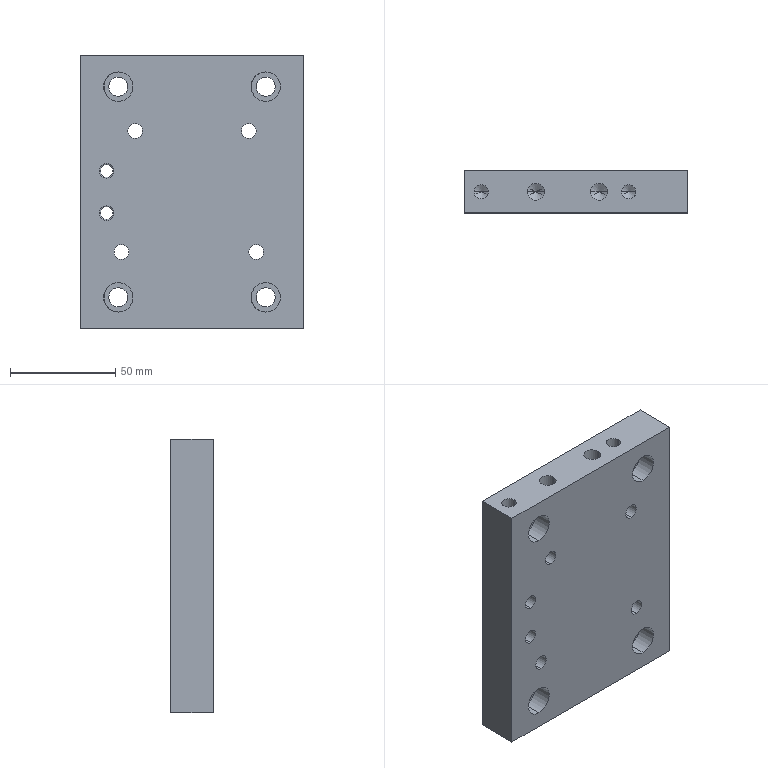Part | STEP file | OP10-149_base block (upper)-L | 1 solid | 92 faces | box 106 x 20 x 130 mm | volume 253956 mm3 | cylinder 56 | cone 20 | plane 16 | commonest cylinder face diameters 6.8 x12 7 x8 8 x8 9 x8 11 x8 14 x8